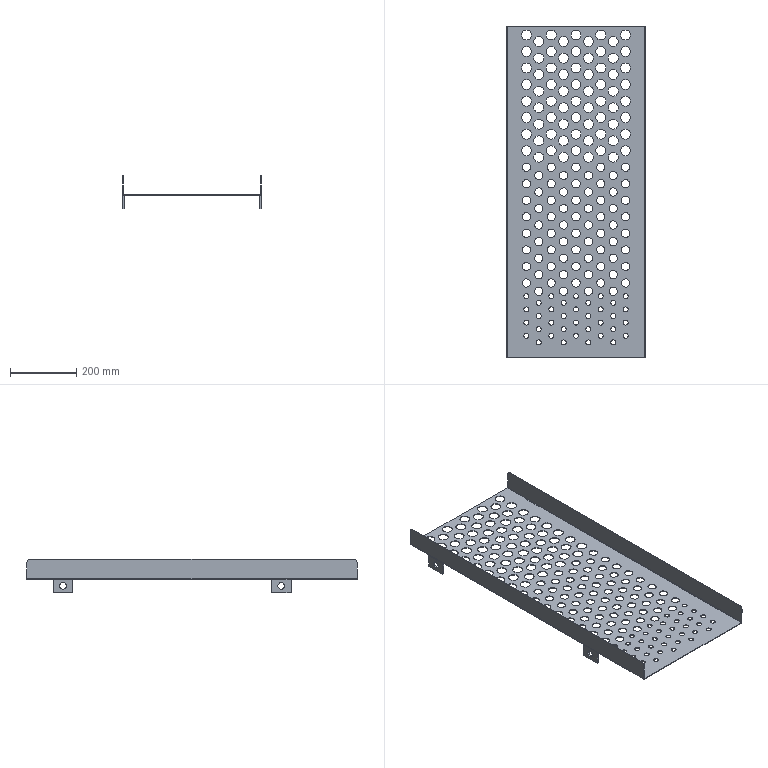Part | SolidWorks | features ICE 8, LPattern 6, EdgeFlange 1, Fillet 1, FlatPattern 1, MirrorPattern 1, SMBaseFlange 1, SheetMetal 1 | 1 solid | 418 faces | box 420 x 1000 x 100 mm | volume 925367 mm3 | cylinder 376 | plane 42 | commonest cylinder face diameters 25 x144 30 x144 15 x72 20 x12 1.473 x2 5.473 x2